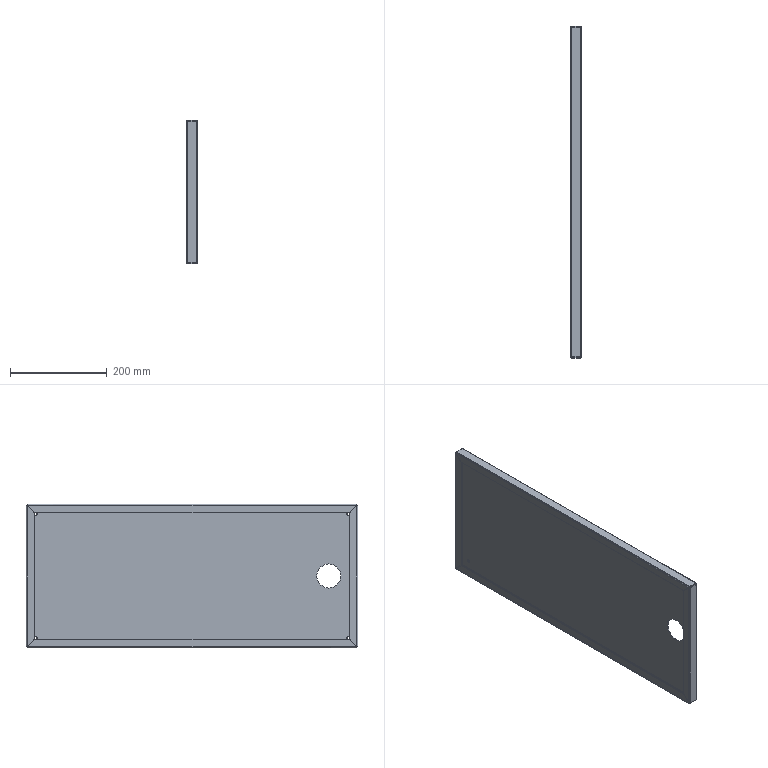Part | STEP file | PN_0075 front door | 1 solid | 80 faces | box 21.5 x 687 x 297 mm | volume 402956 mm3 | plane 38 | cylinder 26 | spline 16 | commonest cylinder face diameters 1.473 x8 4.473 x8 6 x8 50 x2